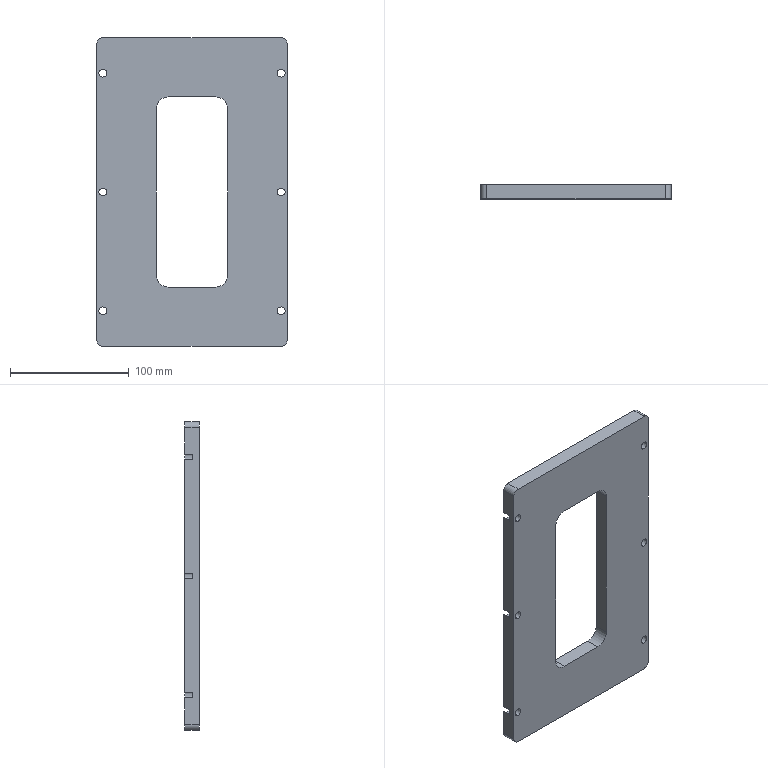Part | STEP file | PN_0008 | 1 solid | 54 faces | box 160 x 12 x 260 mm | volume 379891 mm3 | cylinder 38 | plane 16 | commonest cylinder face diameters 11 x18 6.6 x12 10 x4 20 x4